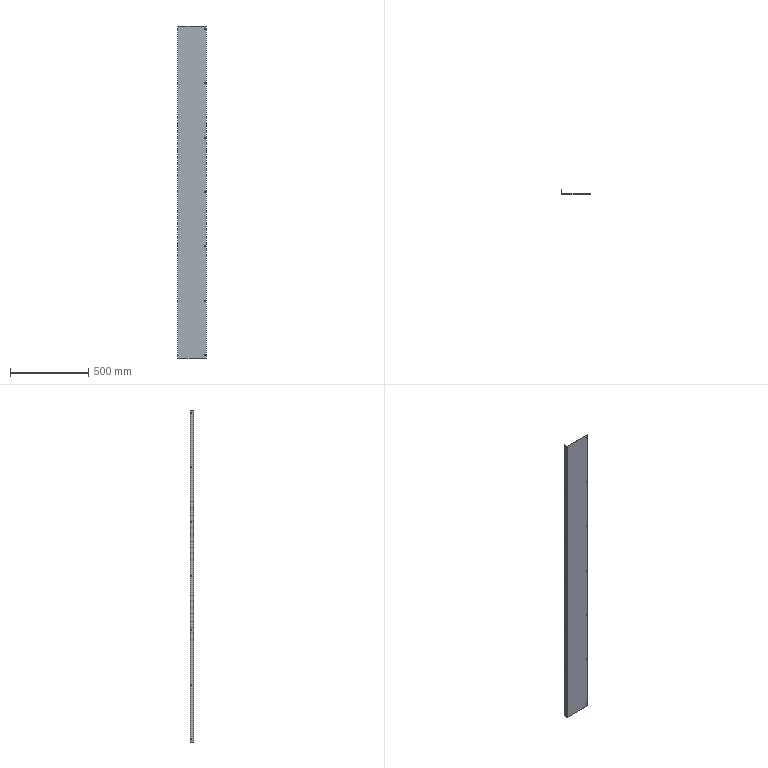Part | SolidWorks | features ICE 2, FlatPattern 1, SMBaseFlange 1, SheetMetal 1 | 1 solid | 70 faces | box 184 x 24 x 2116 mm | volume 436728 mm3 | plane 40 | cylinder 30 | commonest cylinder face diameters 6 x28 0.4 x1 2.4 x1